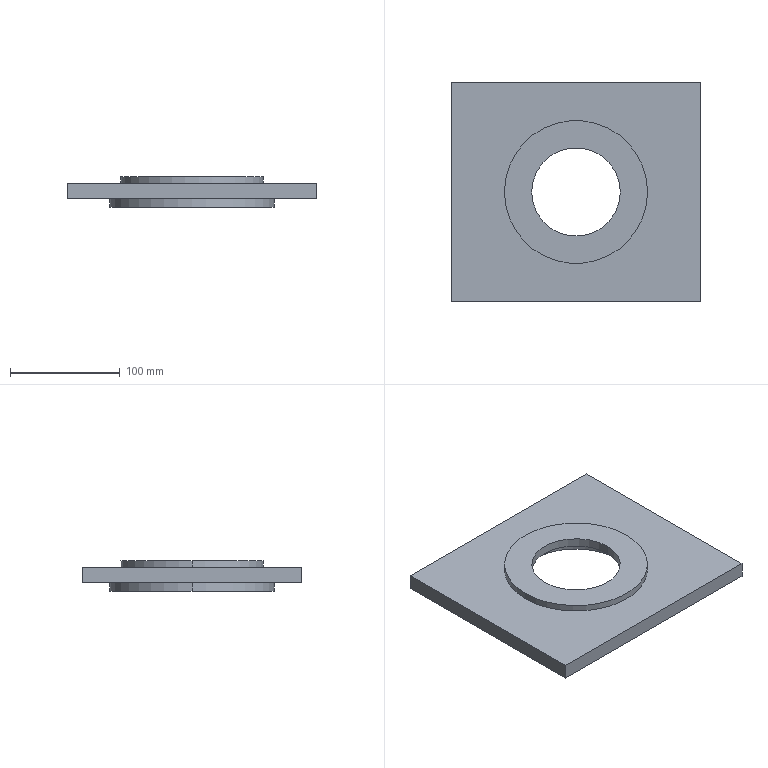Part | SolidWorks | features ICE 4, Extrusion 1 | 1 solid | 20 faces | box 227 x 200 x 28 mm | volume 588836 mm3 | cylinder 10 | plane 10 | commonest cylinder face diameters 80.5 x2 105 x2 130 x2 140 x2 150 x2
STEP:
#1=CARTESIAN_POINT('',(166.,100.,12.));
#2=VERTEX_POINT('',#1);
#3=CARTESIAN_POINT('',(61.,100.,12.));
#4=VERTEX_POINT('',#3);
#5=CARTESIAN_POINT('',(113.5,100.,12.));
#6=DIRECTION('',(0.,0.,-1.));
#7=DIRECTION('',(-1.,0.,0.));
#8=AXIS2_PLACEMENT_3D('',#5,#6,#7);
#9=CIRCLE('',#8,52.5);
#10=EDGE_CURVE('',#2,#4,#9,.T.);
#11=ORIENTED_EDGE('',*,*,#10,.F.);
#12=CARTESIAN_POINT('',(166.,100.,0.));
#13=VERTEX_POINT('',#12);
#14=CARTESIAN_POINT('',(166.,100.,12.));
#15=DIRECTION('',(0.,0.,-1.));
#16=VECTOR('',#15,1000.);
#17=LINE('',#14,#16);
#18=EDGE_CURVE('',#2,#13,#17,.T.);
#19=ORIENTED_EDGE('',*,*,#18,.T.);
#20=CARTESIAN_POINT('',(61.,100.,0.));
#21=VERTEX_POINT('',#20);
#22=CARTESIAN_POINT('',(113.5,100.,0.));
#23=DIRECTION('',(0.,0.,-1.));
#24=DIRECTION('',(-1.,0.,0.));
#25=AXIS2_PLACEMENT_3D('',#22,#23,#24);
#26=CIRCLE('',#25,52.5);
#27=EDGE_CURVE('',#13,#21,#26,.T.);
#28=ORIENTED_EDGE('',*,*,#27,.T.);
#29=CARTESIAN_POINT('',(61.,100.,12.));
#30=DIRECTION('',(0.,0.,-1.));
#31=VECTOR('',#30,1000.);
#32=LINE('',#29,#31);
#33=EDGE_CURVE('',#4,#21,#32,.T.);
#34=ORIENTED_EDGE('',*,*,#33,.F.);
#35=EDGE_LOOP('',(#11,#19,#28,#34));
#36=FACE_OUTER_BOUND('',#35,.T.);
#37=CARTESIAN_POINT('',(113.5,100.,12.));
#38=DIRECTION('',(0.,0.,-1.));
#39=DIRECTION('',(-1.,0.,0.));
#40=AXIS2_PLACEMENT_3D('',#37,#38,#39);
#41=CYLINDRICAL_SURFACE('',#40,52.5);
#42=ADVANCED_FACE('',(#36),#41,.F.);
#43=CARTESIAN_POINT('',(183.5,100.,-8.));
#44=VERTEX_POINT('',#43);
#45=CARTESIAN_POINT('',(43.5,100.,-8.));
#46=VERTEX_POINT('',#45);
#47=CARTESIAN_POINT('',(113.5,100.,-8.));
#48=DIRECTION('',(0.,0.,-1.));
#49=DIRECTION('',(-1.,0.,0.));
#50=AXIS2_PLACEMENT_3D('',#47,#48,#49);
#51=CIRCLE('',#50,70.);
#52=EDGE_CURVE('',#44,#46,#51,.T.);
#53=ORIENTED_EDGE('',*,*,#52,.T.);
#54=CARTESIAN_POINT('',(43.5,100.,0.));
#55=VERTEX_POINT('',#54);
#56=CARTESIAN_POINT('',(43.5,100.,-8.));
#57=DIRECTION('',(0.,0.,1.));
#58=VECTOR('',#57,1000.);
#59=LINE('',#56,#58);
#60=EDGE_CURVE('',#46,#55,#59,.T.);
#61=ORIENTED_EDGE('',*,*,#60,.T.);
#62=CARTESIAN_POINT('',(183.5,100.,0.));
#63=VERTEX_POINT('',#62);
#64=CARTESIAN_POINT('',(113.5,100.,0.));
#65=DIRECTION('',(0.,0.,1.));
#66=DIRECTION('',(-1.,0.,0.));
#67=AXIS2_PLACEMENT_3D('',#64,#65,#66);
#68=CIRCLE('',#67,70.);
#69=EDGE_CURVE('',#55,#63,#68,.T.);
#70=ORIENTED_EDGE('',*,*,#69,.T.);
#71=CARTESIAN_POINT('',(183.5,100.,-8.));
#72=DIRECTION('',(0.,0.,1.));
#73=VECTOR('',#72,1000.);
#74=LINE('',#71,#73);
#75=EDGE_CURVE('',#44,#63,#74,.T.);
#76=ORIENTED_EDGE('',*,*,#75,.F.);
#77=EDGE_LOOP('',(#53,#61,#70,#76));
#78=FACE_OUTER_BOUND('',#77,.T.);
#79=CARTESIAN_POINT('',(113.5,100.,-8.));
#80=DIRECTION('',(0.,0.,1.));
#81=DIRECTION('',(1.,0.,0.));
#82=AXIS2_PLACEMENT_3D('',#79,#80,#81);
#83=CYLINDRICAL_SURFACE('',#82,70.);
#84=ADVANCED_FACE('',(#78),#83,.F.);
#85=CARTESIAN_POINT('',(38.5,100.,-8.));
#86=VERTEX_POINT('',#85);
#87=CARTESIAN_POINT('',(188.5,100.,-8.));
#88=VERTEX_POINT('',#87);
#89=CARTESIAN_POINT('',(113.5,100.,-8.));
#90=DIRECTION('',(0.,0.,-1.));
#91=DIRECTION('',(-1.,0.,0.));
#92=AXIS2_PLACEMENT_3D('',#89,#90,#91);
#93=CIRCLE('',#92,75.);
#94=EDGE_CURVE('',#86,#88,#93,.T.);
#95=ORIENTED_EDGE('',*,*,#94,.F.);
#96=CARTESIAN_POINT('',(38.5,100.,0.));
#97=VERTEX_POINT('',#96);
#98=CARTESIAN_POINT('',(38.5,100.,-8.));
#99=DIRECTION('',(0.,0.,1.));
#100=VECTOR('',#99,1000.);
#101=LINE('',#98,#100);
#102=EDGE_CURVE('',#86,#97,#101,.T.);
#103=ORIENTED_EDGE('',*,*,#102,.T.);
#104=CARTESIAN_POINT('',(188.5,100.,0.));
#105=VERTEX_POINT('',#104);
#106=CARTESIAN_POINT('',(113.5,100.,0.));
#107=DIRECTION('',(0.,0.,-1.));
#108=DIRECTION('',(-1.,0.,0.));
#109=AXIS2_PLACEMENT_3D('',#106,#107,#108);
#110=CIRCLE('',#109,75.);
#111=EDGE_CURVE('',#97,#105,#110,.T.);
#112=ORIENTED_EDGE('',*,*,#111,.T.);
#113=CARTESIAN_POINT('',(188.5,100.,-8.));
#114=DIRECTION('',(0.,0.,1.));
#115=VECTOR('',#114,1000.);
#116=LINE('',#113,#115);
#117=EDGE_CURVE('',#88,#105,#116,.T.);
#118=ORIENTED_EDGE('',*,*,#117,.F.);
#119=EDGE_LOOP('',(#95,#103,#112,#118));
#120=FACE_OUTER_BOUND('',#119,.T.);
#121=CARTESIAN_POINT('',(113.5,100.,-8.));
#122=DIRECTION('',(0.,0.,1.));
#123=DIRECTION('',(1.,0.,0.));
#124=AXIS2_PLACEMENT_3D('',#121,#122,#123);
#125=CYLINDRICAL_SURFACE('',#124,75.);
#126=ADVANCED_FACE('',(#120),#125,.T.);
#127=CARTESIAN_POINT('',(178.5,100.,20.));
#128=VERTEX_POINT('',#127);
#129=CARTESIAN_POINT('',(48.5,100.,20.));
#130=VERTEX_POINT('',#129);
#131=CARTESIAN_POINT('',(113.5,100.,20.));
#132=DIRECTION('',(0.,0.,1.));
#133=DIRECTION('',(1.,0.,0.));
#134=AXIS2_PLACEMENT_3D('',#131,#132,#133);
#135=CIRCLE('',#134,65.);
#136=EDGE_CURVE('',#128,#130,#135,.T.);
#137=ORIENTED_EDGE('',*,*,#136,.F.);
#138=CARTESIAN_POINT('',(178.5,100.,14.));
#139=VERTEX_POINT('',#138);
#140=CARTESIAN_POINT('',(178.5,100.,20.));
#141=DIRECTION('',(0.,0.,-1.));
#142=VECTOR('',#141,1000.);
#143=LINE('',#140,#142);
#144=EDGE_CURVE('',#128,#139,#143,.T.);
#145=ORIENTED_EDGE('',*,*,#144,.T.);
#146=CARTESIAN_POINT('',(48.5,100.,14.));
#147=VERTEX_POINT('',#146);
#148=CARTESIAN_POINT('',(113.5,100.,14.));
#149=DIRECTION('',(0.,0.,1.));
#150=DIRECTION('',(-1.,0.,0.));
#151=AXIS2_PLACEMENT_3D('',#148,#149,#150);
#152=CIRCLE('',#151,65.);
#153=EDGE_CURVE('',#139,#147,#152,.T.);
#154=ORIENTED_EDGE('',*,*,#153,.T.);
#155=CARTESIAN_POINT('',(48.5,100.,20.));
#156=DIRECTION('',(0.,0.,-1.));
#157=VECTOR('',#156,1000.);
#158=LINE('',#155,#157);
#159=EDGE_CURVE('',#130,#147,#158,.T.);
#160=ORIENTED_EDGE('',*,*,#159,.F.);
#161=EDGE_LOOP('',(#137,#145,#154,#160));
#162=FACE_OUTER_BOUND('',#161,.T.);
#163=CARTESIAN_POINT('',(113.5,100.,20.));
#164=DIRECTION('',(0.,0.,-1.));
#165=DIRECTION('',(-1.,0.,0.));
#166=AXIS2_PLACEMENT_3D('',#163,#164,#165);
#167=CYLINDRICAL_SURFACE('',#166,65.);
#168=ADVANCED_FACE('',(#162),#167,.T.);
#169=CARTESIAN_POINT('',(73.25,100.,12.));
#170=VERTEX_POINT('',#169);
#171=CARTESIAN_POINT('',(153.75,100.,12.));
#172=VERTEX_POINT('',#171);
#173=CARTESIAN_POINT('',(113.5,100.,12.));
#174=DIRECTION('',(0.,0.,1.));
#175=DIRECTION('',(-1.,0.,0.));
#176=AXIS2_PLACEMENT_3D('',#173,#174,#175);
#177=CIRCLE('',#176,40.25);
#178=EDGE_CURVE('',#170,#172,#177,.T.);
#179=ORIENTED_EDGE('',*,*,#178,.F.);
#180=CARTESIAN_POINT('',(73.25,100.,20.));
#181=VERTEX_POINT('',#180);
#182=CARTESIAN_POINT('',(73.25,100.,-8.));
#183=DIRECTION('',(0.,0.,1.));
#184=VECTOR('',#183,1000.);
#185=LINE('',#182,#184);
#186=EDGE_CURVE('',#170,#181,#185,.T.);
#187=ORIENTED_EDGE('',*,*,#186,.T.);
#188=CARTESIAN_POINT('',(153.75,100.,20.));
#189=VERTEX_POINT('',#188);
#190=CARTESIAN_POINT('',(113.5,100.,20.));
#191=DIRECTION('',(0.,0.,1.));
#192=DIRECTION('',(1.,0.,0.));
#193=AXIS2_PLACEMENT_3D('',#190,#191,#192);
#194=CIRCLE('',#193,40.25);
#195=EDGE_CURVE('',#181,#189,#194,.T.);
#196=ORIENTED_EDGE('',*,*,#195,.T.);
#197=CARTESIAN_POINT('',(153.75,100.,-8.));
#198=DIRECTION('',(0.,0.,1.));
#199=VECTOR('',#198,1000.);
#200=LINE('',#197,#199);
#201=EDGE_CURVE('',#172,#189,#200,.T.);
#202=ORIENTED_EDGE('',*,*,#201,.F.);
#203=EDGE_LOOP('',(#179,#187,#196,#202));
#204=FACE_OUTER_BOUND('',#203,.T.);
#205=CARTESIAN_POINT('',(113.5,100.,-8.));
#206=DIRECTION('',(0.,0.,1.));
#207=DIRECTION('',(1.,0.,0.));
#208=AXIS2_PLACEMENT_3D('',#205,#206,#207);
#209=CYLINDRICAL_SURFACE('',#208,40.25);
#210=ADVANCED_FACE('',(#204),#209,.F.);
#211=ORIENTED_EDGE('',*,*,#186,.F.);
#212=CARTESIAN_POINT('',(113.5,100.,12.));
#213=DIRECTION('',(0.,0.,1.));
#214=DIRECTION('',(-1.,0.,0.));
#215=AXIS2_PLACEMENT_3D('',#212,#213,#214);
#216=CIRCLE('',#215,40.25);
#217=EDGE_CURVE('',#172,#170,#216,.T.);
#218=ORIENTED_EDGE('',*,*,#217,.F.);
#219=ORIENTED_EDGE('',*,*,#201,.T.);
#220=CARTESIAN_POINT('',(113.5,100.,20.));
#221=DIRECTION('',(0.,0.,1.));
#222=DIRECTION('',(1.,0.,0.));
#223=AXIS2_PLACEMENT_3D('',#220,#221,#222);
#224=CIRCLE('',#223,40.25);
#225=EDGE_CURVE('',#189,#181,#224,.T.);
#226=ORIENTED_EDGE('',*,*,#225,.T.);
#227=EDGE_LOOP('',(#211,#218,#219,#226));
#228=FACE_OUTER_BOUND('',#227,.T.);
#229=CARTESIAN_POINT('',(113.5,100.,-8.));
#230=DIRECTION('',(0.,0.,1.));
#231=DIRECTION('',(1.,0.,0.));
#232=AXIS2_PLACEMENT_3D('',#229,#230,#231);
#233=CYLINDRICAL_SURFACE('',#232,40.25);
#234=ADVANCED_FACE('',(#228),#233,.F.);
#235=CARTESIAN_POINT('',(0.,0.,0.));
#236=VERTEX_POINT('',#235);
#237=CARTESIAN_POINT('',(227.,0.,0.));
#238=VERTEX_POINT('',#237);
#239=CARTESIAN_POINT('',(227.,0.,0.));
#240=DIRECTION('',(1.,0.,0.));
#241=VECTOR('',#240,1000.);
#242=LINE('',#239,#241);
#243=EDGE_CURVE('',#236,#238,#242,.T.);
#244=ORIENTED_EDGE('',*,*,#243,.F.);
#245=CARTESIAN_POINT('',(0.,200.,0.));
#246=VERTEX_POINT('',#245);
#247=CARTESIAN_POINT('',(0.,0.,0.));
#248=DIRECTION('',(0.,-1.,0.));
#249=VECTOR('',#248,1000.);
#250=LINE('',#247,#249);
#251=EDGE_CURVE('',#246,#236,#250,.T.);
#252=ORIENTED_EDGE('',*,*,#251,.F.);
#253=CARTESIAN_POINT('',(227.,200.,0.));
#254=VERTEX_POINT('',#253);
#255=CARTESIAN_POINT('',(0.,200.,0.));
#256=DIRECTION('',(-1.,0.,0.));
#257=VECTOR('',#256,1000.);
#258=LINE('',#255,#257);
#259=EDGE_CURVE('',#254,#246,#258,.T.);
#260=ORIENTED_EDGE('',*,*,#259,.F.);
#261=CARTESIAN_POINT('',(227.,200.,0.));
#262=DIRECTION('',(0.,1.,0.));
#263=VECTOR('',#262,1000.);
#264=LINE('',#261,#263);
#265=EDGE_CURVE('',#238,#254,#264,.T.);
#266=ORIENTED_EDGE('',*,*,#265,.F.);
#267=EDGE_LOOP('',(#244,#252,#260,#266));
#268=FACE_OUTER_BOUND('',#267,.T.);
#269=CARTESIAN_POINT('',(113.5,100.,0.));
#270=DIRECTION('',(0.,0.,-1.));
#271=DIRECTION('',(-1.,0.,0.));
#272=AXIS2_PLACEMENT_3D('',#269,#270,#271);
#273=CIRCLE('',#272,75.);
#274=EDGE_CURVE('',#105,#97,#273,.T.);
#275=ORIENTED_EDGE('',*,*,#274,.F.);
#276=ORIENTED_EDGE('',*,*,#111,.F.);
#277=EDGE_LOOP('',(#275,#276));
#278=FACE_BOUND('',#277,.T.);
#279=CARTESIAN_POINT('',(0.,0.,0.));
#280=DIRECTION('',(0.,0.,-1.));
#281=DIRECTION('',(-1.,0.,0.));
#282=AXIS2_PLACEMENT_3D('',#279,#280,#281);
#283=PLANE('',#282);
#284=ADVANCED_FACE('',(#268,#278),#283,.T.);
#285=CARTESIAN_POINT('',(0.,0.,14.));
#286=VERTEX_POINT('',#285);
#287=CARTESIAN_POINT('',(227.,0.,14.));
#288=VERTEX_POINT('',#287);
#289=CARTESIAN_POINT('',(227.,0.,14.));
#290=DIRECTION('',(1.,0.,0.));
#291=VECTOR('',#290,1000.);
#292=LINE('',#289,#291);
#293=EDGE_CURVE('',#286,#288,#292,.T.);
#294=ORIENTED_EDGE('',*,*,#293,.T.);
#295=CARTESIAN_POINT('',(227.,200.,14.));
#296=VERTEX_POINT('',#295);
#297=CARTESIAN_POINT('',(227.,200.,14.));
#298=DIRECTION('',(0.,1.,0.));
#299=VECTOR('',#298,1000.);
#300=LINE('',#297,#299);
#301=EDGE_CURVE('',#288,#296,#300,.T.);
#302=ORIENTED_EDGE('',*,*,#301,.T.);
#303=CARTESIAN_POINT('',(0.,200.,14.));
#304=VERTEX_POINT('',#303);
#305=CARTESIAN_POINT('',(0.,200.,14.));
#306=DIRECTION('',(-1.,0.,0.));
#307=VECTOR('',#306,1000.);
#308=LINE('',#305,#307);
#309=EDGE_CURVE('',#296,#304,#308,.T.);
#310=ORIENTED_EDGE('',*,*,#309,.T.);
#311=CARTESIAN_POINT('',(0.,0.,14.));
#312=DIRECTION('',(0.,-1.,0.));
#313=VECTOR('',#312,1000.);
#314=LINE('',#311,#313);
#315=EDGE_CURVE('',#304,#286,#314,.T.);
#316=ORIENTED_EDGE('',*,*,#315,.T.);
#317=EDGE_LOOP('',(#294,#302,#310,#316));
#318=FACE_OUTER_BOUND('',#317,.T.);
#319=CARTESIAN_POINT('',(113.5,100.,14.));
#320=DIRECTION('',(0.,0.,1.));
#321=DIRECTION('',(-1.,0.,0.));
#322=AXIS2_PLACEMENT_3D('',#319,#320,#321);
#323=CIRCLE('',#322,65.);
#324=EDGE_CURVE('',#147,#139,#323,.T.);
#325=ORIENTED_EDGE('',*,*,#324,.F.);
#326=ORIENTED_EDGE('',*,*,#153,.F.);
#327=EDGE_LOOP('',(#325,#326));
#328=FACE_BOUND('',#327,.T.);
#329=CARTESIAN_POINT('',(0.,0.,14.));
#330=DIRECTION('',(0.,0.,-1.));
#331=DIRECTION('',(-1.,0.,0.));
#332=AXIS2_PLACEMENT_3D('',#329,#330,#331);
#333=PLANE('',#332);
#334=ADVANCED_FACE('',(#318,#328),#333,.F.);
#335=ORIENTED_EDGE('',*,*,#243,.T.);
#336=CARTESIAN_POINT('',(227.,0.,14.));
#337=DIRECTION('',(0.,0.,-1.));
#338=VECTOR('',#337,1000.);
#339=LINE('',#336,#338);
#340=EDGE_CURVE('',#288,#238,#339,.T.);
#341=ORIENTED_EDGE('',*,*,#340,.F.);
#342=ORIENTED_EDGE('',*,*,#293,.F.);
#343=CARTESIAN_POINT('',(0.,0.,14.));
#344=DIRECTION('',(0.,0.,-1.));
#345=VECTOR('',#344,1000.);
#346=LINE('',#343,#345);
#347=EDGE_CURVE('',#286,#236,#346,.T.);
#348=ORIENTED_EDGE('',*,*,#347,.T.);
#349=EDGE_LOOP('',(#335,#341,#342,#348));
#350=FACE_OUTER_BOUND('',#349,.T.);
#351=CARTESIAN_POINT('',(227.,0.,14.));
#352=DIRECTION('',(0.,1.,0.));
#353=DIRECTION('',(-1.,0.,0.));
#354=AXIS2_PLACEMENT_3D('',#351,#352,#353);
#355=PLANE('',#354);
#356=ADVANCED_FACE('',(#350),#355,.F.);
#357=ORIENTED_EDGE('',*,*,#265,.T.);
#358=CARTESIAN_POINT('',(227.,200.,14.));
#359=DIRECTION('',(0.,0.,-1.));
#360=VECTOR('',#359,1000.);
#361=LINE('',#358,#360);
#362=EDGE_CURVE('',#296,#254,#361,.T.);
#363=ORIENTED_EDGE('',*,*,#362,.F.);
#364=ORIENTED_EDGE('',*,*,#301,.F.);
#365=ORIENTED_EDGE('',*,*,#340,.T.);
#366=EDGE_LOOP('',(#357,#363,#364,#365));
#367=FACE_OUTER_BOUND('',#366,.T.);
#368=CARTESIAN_POINT('',(227.,200.,14.));
#369=DIRECTION('',(-1.,0.,0.));
#370=DIRECTION('',(0.,-1.,0.));
#371=AXIS2_PLACEMENT_3D('',#368,#369,#370);
#372=PLANE('',#371);
#373=ADVANCED_FACE('',(#367),#372,.F.);
#374=ORIENTED_EDGE('',*,*,#259,.T.);
#375=CARTESIAN_POINT('',(0.,200.,14.));
#376=DIRECTION('',(0.,0.,-1.));
#377=VECTOR('',#376,1000.);
#378=LINE('',#375,#377);
#379=EDGE_CURVE('',#304,#246,#378,.T.);
#380=ORIENTED_EDGE('',*,*,#379,.F.);
#381=ORIENTED_EDGE('',*,*,#309,.F.);
#382=ORIENTED_EDGE('',*,*,#362,.T.);
#383=EDGE_LOOP('',(#374,#380,#381,#382));
#384=FACE_OUTER_BOUND('',#383,.T.);
#385=CARTESIAN_POINT('',(0.,200.,14.));
#386=DIRECTION('',(0.,-1.,0.));
#387=DIRECTION('',(0.,0.,-1.));
#388=AXIS2_PLACEMENT_3D('',#385,#386,#387);
#389=PLANE('',#388);
#390=ADVANCED_FACE('',(#384),#389,.F.);
#391=ORIENTED_EDGE('',*,*,#251,.T.);
#392=ORIENTED_EDGE('',*,*,#347,.F.);
#393=ORIENTED_EDGE('',*,*,#315,.F.);
#394=ORIENTED_EDGE('',*,*,#379,.T.);
#395=EDGE_LOOP('',(#391,#392,#393,#394));
#396=FACE_OUTER_BOUND('',#395,.T.);
#397=CARTESIAN_POINT('',(0.,0.,14.));
#398=DIRECTION('',(1.,0.,0.));
#399=DIRECTION('',(0.,0.,-1.));
#400=AXIS2_PLACEMENT_3D('',#397,#398,#399);
#401=PLANE('',#400);
#402=ADVANCED_FACE('',(#396),#401,.F.);
#403=ORIENTED_EDGE('',*,*,#144,.F.);
#404=CARTESIAN_POINT('',(113.5,100.,20.));
#405=DIRECTION('',(0.,0.,1.));
#406=DIRECTION('',(1.,0.,0.));
#407=AXIS2_PLACEMENT_3D('',#404,#405,#406);
#408=CIRCLE('',#407,65.);
#409=EDGE_CURVE('',#130,#128,#408,.T.);
#410=ORIENTED_EDGE('',*,*,#409,.F.);
#411=ORIENTED_EDGE('',*,*,#159,.T.);
#412=ORIENTED_EDGE('',*,*,#324,.T.);
#413=EDGE_LOOP('',(#403,#410,#411,#412));
#414=FACE_OUTER_BOUND('',#413,.T.);
#415=CARTESIAN_POINT('',(113.5,100.,20.));
#416=DIRECTION('',(0.,0.,-1.));
#417=DIRECTION('',(-1.,0.,0.));
#418=AXIS2_PLACEMENT_3D('',#415,#416,#417);
#419=CYLINDRICAL_SURFACE('',#418,65.);
#420=ADVANCED_FACE('',(#414),#419,.T.);
#421=ORIENTED_EDGE('',*,*,#225,.F.);
#422=ORIENTED_EDGE('',*,*,#195,.F.);
#423=EDGE_LOOP('',(#421,#422));
#424=FACE_BOUND('',#423,.T.);
#425=ORIENTED_EDGE('',*,*,#409,.T.);
#426=ORIENTED_EDGE('',*,*,#136,.T.);
#427=EDGE_LOOP('',(#425,#426));
#428=FACE_OUTER_BOUND('',#427,.T.);
#429=CARTESIAN_POINT('',(113.5,100.,20.));
#430=DIRECTION('',(0.,0.,1.));
#431=DIRECTION('',(1.,0.,0.));
#432=AXIS2_PLACEMENT_3D('',#429,#430,#431);
#433=PLANE('',#432);
#434=ADVANCED_FACE('',(#424,#428),#433,.T.);
#435=CARTESIAN_POINT('',(113.5,100.,-8.));
#436=DIRECTION('',(0.,0.,-1.));
#437=DIRECTION('',(-1.,0.,0.));
#438=AXIS2_PLACEMENT_3D('',#435,#436,#437);
#439=CIRCLE('',#438,75.);
#440=EDGE_CURVE('',#88,#86,#439,.T.);
#441=ORIENTED_EDGE('',*,*,#440,.T.);
#442=ORIENTED_EDGE('',*,*,#94,.T.);
#443=EDGE_LOOP('',(#441,#442));
#444=FACE_OUTER_BOUND('',#443,.T.);
#445=ORIENTED_EDGE('',*,*,#52,.F.);
#446=CARTESIAN_POINT('',(113.5,100.,-8.));
#447=DIRECTION('',(0.,0.,-1.));
#448=DIRECTION('',(-1.,0.,0.));
#449=AXIS2_PLACEMENT_3D('',#446,#447,#448);
#450=CIRCLE('',#449,70.);
#451=EDGE_CURVE('',#46,#44,#450,.T.);
#452=ORIENTED_EDGE('',*,*,#451,.F.);
#453=EDGE_LOOP('',(#445,#452));
#454=FACE_BOUND('',#453,.T.);
#455=CARTESIAN_POINT('',(113.5,100.,-8.));
#456=DIRECTION('',(0.,0.,-1.));
#457=DIRECTION('',(-1.,0.,0.));
#458=AXIS2_PLACEMENT_3D('',#455,#456,#457);
#459=PLANE('',#458);
#460=ADVANCED_FACE('',(#444,#454),#459,.T.);
#461=ORIENTED_EDGE('',*,*,#102,.F.);
#462=ORIENTED_EDGE('',*,*,#440,.F.);
#463=ORIENTED_EDGE('',*,*,#117,.T.);
#464=ORIENTED_EDGE('',*,*,#274,.T.);
#465=EDGE_LOOP('',(#461,#462,#463,#464));
#466=FACE_OUTER_BOUND('',#465,.T.);
#467=CARTESIAN_POINT('',(113.5,100.,-8.));
#468=DIRECTION('',(0.,0.,1.));
#469=DIRECTION('',(1.,0.,0.));
#470=AXIS2_PLACEMENT_3D('',#467,#468,#469);
#471=CYLINDRICAL_SURFACE('',#470,75.);
#472=ADVANCED_FACE('',(#466),#471,.T.);
#473=ORIENTED_EDGE('',*,*,#60,.F.);
#474=ORIENTED_EDGE('',*,*,#451,.T.);
#475=ORIENTED_EDGE('',*,*,#75,.T.);
#476=CARTESIAN_POINT('',(113.5,100.,0.));
#477=DIRECTION('',(0.,0.,1.));
#478=DIRECTION('',(-1.,0.,0.));
#479=AXIS2_PLACEMENT_3D('',#476,#477,#478);
#480=CIRCLE('',#479,70.);
#481=EDGE_CURVE('',#63,#55,#480,.T.);
#482=ORIENTED_EDGE('',*,*,#481,.T.);
#483=EDGE_LOOP('',(#473,#474,#475,#482));
#484=FACE_OUTER_BOUND('',#483,.T.);
#485=CARTESIAN_POINT('',(113.5,100.,-8.));
#486=DIRECTION('',(0.,0.,1.));
#487=DIRECTION('',(1.,0.,0.));
#488=AXIS2_PLACEMENT_3D('',#485,#486,#487);
#489=CYLINDRICAL_SURFACE('',#488,70.);
#490=ADVANCED_FACE('',(#484),#489,.F.);
#491=CARTESIAN_POINT('',(113.5,100.,0.));
#492=DIRECTION('',(0.,0.,-1.));
#493=DIRECTION('',(-1.,0.,0.));
#494=AXIS2_PLACEMENT_3D('',#491,#492,#493);
#495=CIRCLE('',#494,52.5);
#496=EDGE_CURVE('',#21,#13,#495,.T.);
#497=ORIENTED_EDGE('',*,*,#496,.F.);
#498=ORIENTED_EDGE('',*,*,#27,.F.);
#499=EDGE_LOOP('',(#497,#498));
#500=FACE_BOUND('',#499,.T.);
#501=ORIENTED_EDGE('',*,*,#481,.F.);
#502=ORIENTED_EDGE('',*,*,#69,.F.);
#503=EDGE_LOOP('',(#501,#502));
#504=FACE_OUTER_BOUND('',#503,.T.);
#505=CARTESIAN_POINT('',(0.,0.,0.));
#506=DIRECTION('',(0.,0.,-1.));
#507=DIRECTION('',(-1.,0.,0.));
#508=AXIS2_PLACEMENT_3D('',#505,#506,#507);
#509=PLANE('',#508);
#510=ADVANCED_FACE('',(#500,#504),#509,.T.);
#511=CARTESIAN_POINT('',(113.5,100.,12.));
#512=DIRECTION('',(0.,0.,-1.));
#513=DIRECTION('',(-1.,0.,0.));
#514=AXIS2_PLACEMENT_3D('',#511,#512,#513);
#515=CIRCLE('',#514,52.5);
#516=EDGE_CURVE('',#4,#2,#515,.T.);
#517=ORIENTED_EDGE('',*,*,#516,.T.);
#518=ORIENTED_EDGE('',*,*,#10,.T.);
#519=EDGE_LOOP('',(#517,#518));
#520=FACE_OUTER_BOUND('',#519,.T.);
#521=ORIENTED_EDGE('',*,*,#217,.T.);
#522=ORIENTED_EDGE('',*,*,#178,.T.);
#523=EDGE_LOOP('',(#521,#522));
#524=FACE_BOUND('',#523,.T.);
#525=CARTESIAN_POINT('',(113.5,100.,12.));
#526=DIRECTION('',(0.,0.,-1.));
#527=DIRECTION('',(-1.,0.,0.));
#528=AXIS2_PLACEMENT_3D('',#525,#526,#527);
#529=PLANE('',#528);
#530=ADVANCED_FACE('',(#520,#524),#529,.T.);
#531=ORIENTED_EDGE('',*,*,#18,.F.);
#532=ORIENTED_EDGE('',*,*,#516,.F.);
#533=ORIENTED_EDGE('',*,*,#33,.T.);
#534=ORIENTED_EDGE('',*,*,#496,.T.);
#535=EDGE_LOOP('',(#531,#532,#533,#534));
#536=FACE_OUTER_BOUND('',#535,.T.);
#537=CARTESIAN_POINT('',(113.5,100.,12.));
#538=DIRECTION('',(0.,0.,-1.));
#539=DIRECTION('',(-1.,0.,0.));
#540=AXIS2_PLACEMENT_3D('',#537,#538,#539);
#541=CYLINDRICAL_SURFACE('',#540,52.5);
#542=ADVANCED_FACE('',(#536),#541,.F.);
#543=CLOSED_SHELL('',(#42,#84,#126,#168,#210,#234,#284,#334,#356,#373,#390,#402,#420,#434,#460,#472,#490,#510,#530,#542));
#544=MANIFOLD_SOLID_BREP('',#543);
#545=CARTESIAN_POINT('',(0.,0.,0.));
#546=DIRECTION('',(0.,0.,1.));
#547=DIRECTION('',(1.,0.,0.));
#548=AXIS2_PLACEMENT_3D('',#545,#546,#547);
#549=(LENGTH_UNIT()NAMED_UNIT(*)SI_UNIT(.MILLI.,.METRE.));
#550=UNCERTAINTY_MEASURE_WITH_UNIT(LENGTH_MEASURE(0.00001),#549,'','');
#551=(NAMED_UNIT(*)PLANE_ANGLE_UNIT()SI_UNIT($,.RADIAN.));
#552=(NAMED_UNIT(*)SI_UNIT($,.STERADIAN.)SOLID_ANGLE_UNIT());
#553=(GEOMETRIC_REPRESENTATION_CONTEXT(3)GLOBAL_UNCERTAINTY_ASSIGNED_CONTEXT((#550))GLOBAL_UNIT_ASSIGNED_CONTEXT((#549,#551,#552))REPRESENTATION_CONTEXT('',''));
#554=ADVANCED_BREP_SHAPE_REPRESENTATION('',(#544,#548),#553);